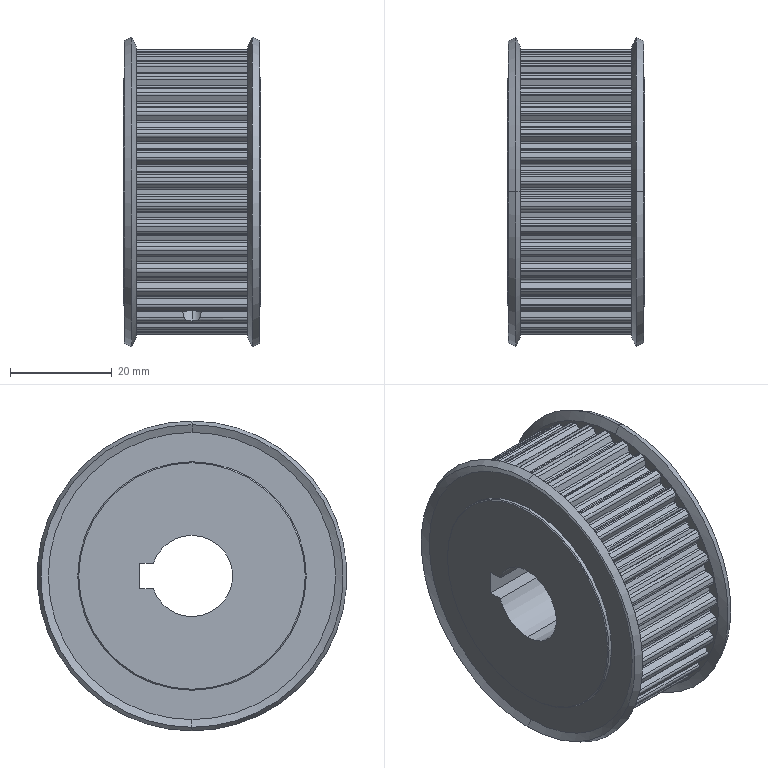Part | SolidWorks | features BaseBody 1 | 1 solid | 366 faces | box 27 x 61 x 61 mm | volume 57588 mm3 | cylinder 267 | plane 85 | cone 14 | commonest cylinder face diameters 0.8 x91 1.2 x90 52.85 x39 56.45 x36 4.134 x4 45 x4